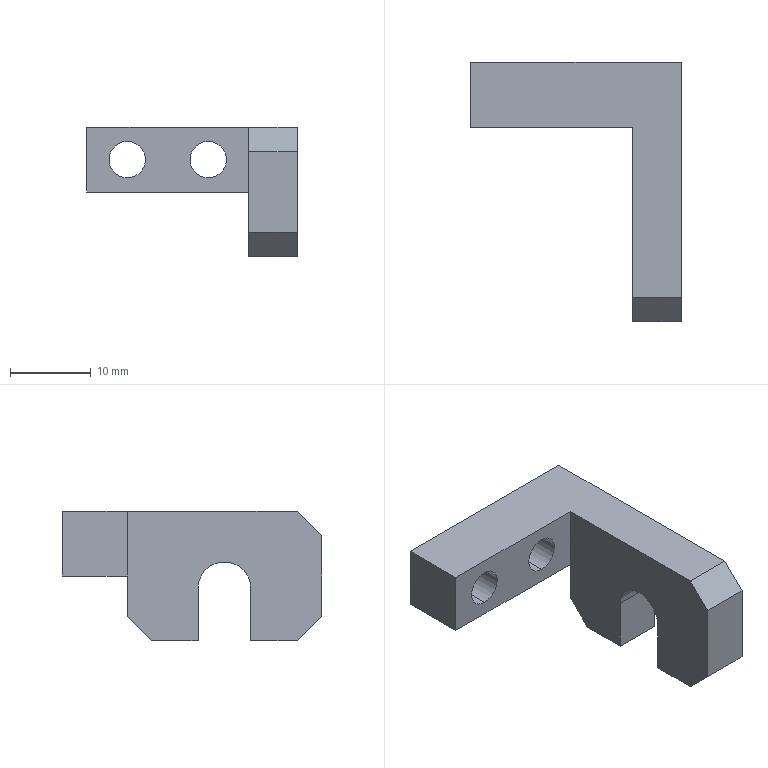Part | STEP file | Product shift cylinder connector | 1 solid | 21 faces | box 26 x 32 x 16 mm | volume 3279 mm3 | plane 16 | cylinder 5 | commonest cylinder face diameters 4.5 x4 6.5 x1